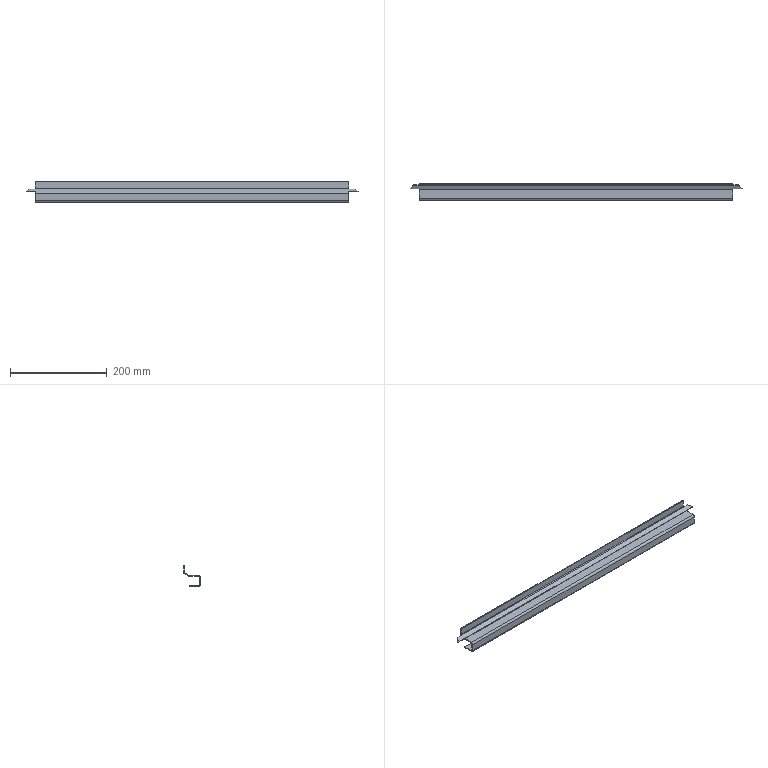Part | NX | features solid 2 | 1 solid | 30 faces | box 687.942 x 35 x 43 mm | volume 117426 mm3 | plane 22 | cylinder 8 | commonest cylinder face diameters 4 x4 8 x4
STEP:
#1=CARTESIAN_POINT('',(1221.029,-650.337,635.595));
#2=VERTEX_POINT('',#1);
#3=CARTESIAN_POINT('',(1228.453,-642.211,639.658));
#4=VERTEX_POINT('',#3);
#5=CARTESIAN_POINT('',(1221.029,-650.337,635.595));
#6=DIRECTION('',(0.6327,0.6926,0.3463));
#7=VECTOR('',#6,1000.);
#8=LINE('',#5,#7);
#9=EDGE_CURVE('',#2,#4,#8,.T.);
#10=ORIENTED_EDGE('',*,*,#9,.F.);
#11=CARTESIAN_POINT('',(1221.029,-651.231,637.384));
#12=VERTEX_POINT('',#11);
#13=CARTESIAN_POINT('',(1221.029,-651.231,637.384));
#14=DIRECTION('',(0.,0.4472,-0.8944));
#15=VECTOR('',#14,1000.);
#16=LINE('',#13,#15);
#17=EDGE_CURVE('',#12,#2,#16,.T.);
#18=ORIENTED_EDGE('',*,*,#17,.F.);
#19=CARTESIAN_POINT('',(1228.453,-643.106,641.447));
#20=VERTEX_POINT('',#19);
#21=CARTESIAN_POINT('',(1221.029,-651.231,637.384));
#22=DIRECTION('',(0.6327,0.6926,0.3463));
#23=VECTOR('',#22,1000.);
#24=LINE('',#21,#23);
#25=EDGE_CURVE('',#12,#20,#24,.T.);
#26=ORIENTED_EDGE('',*,*,#25,.T.);
#27=CARTESIAN_POINT('',(1228.453,-643.106,641.447));
#28=DIRECTION('',(0.,0.4472,-0.8944));
#29=VECTOR('',#28,1000.);
#30=LINE('',#27,#29);
#31=EDGE_CURVE('',#20,#4,#30,.T.);
#32=ORIENTED_EDGE('',*,*,#31,.T.);
#33=EDGE_LOOP('',(#10,#18,#26,#32));
#34=FACE_BOUND('',#33,.T.);
#35=CARTESIAN_POINT('',(1221.029,-651.231,637.384));
#36=DIRECTION('',(-0.7744,0.5659,0.283));
#37=DIRECTION('',(0.3432,0.,0.9393));
#38=AXIS2_PLACEMENT_3D('',#35,#36,#37);
#39=PLANE('',#38);
#40=ADVANCED_FACE('',(#34),#39,.T.);
#41=CARTESIAN_POINT('',(1240.,-650.337,635.595));
#42=VERTEX_POINT('',#41);
#43=CARTESIAN_POINT('',(1240.,-650.337,635.595));
#44=DIRECTION('',(-1.,0.,0.));
#45=VECTOR('',#44,1000.);
#46=LINE('',#43,#45);
#47=EDGE_CURVE('',#42,#2,#46,.T.);
#48=ORIENTED_EDGE('',*,*,#47,.F.);
#49=CARTESIAN_POINT('',(1240.,-651.231,637.384));
#50=VERTEX_POINT('',#49);
#51=CARTESIAN_POINT('',(1240.,-651.231,637.384));
#52=DIRECTION('',(0.,0.4472,-0.8944));
#53=VECTOR('',#52,1000.);
#54=LINE('',#51,#53);
#55=EDGE_CURVE('',#50,#42,#54,.T.);
#56=ORIENTED_EDGE('',*,*,#55,.F.);
#57=CARTESIAN_POINT('',(1240.,-651.231,637.384));
#58=DIRECTION('',(-1.,0.,0.));
#59=VECTOR('',#58,1000.);
#60=LINE('',#57,#59);
#61=EDGE_CURVE('',#50,#12,#60,.T.);
#62=ORIENTED_EDGE('',*,*,#61,.T.);
#63=ORIENTED_EDGE('',*,*,#17,.T.);
#64=EDGE_LOOP('',(#48,#56,#62,#63));
#65=FACE_BOUND('',#64,.T.);
#66=CARTESIAN_POINT('',(1240.,-651.231,637.384));
#67=DIRECTION('',(0.,-0.8944,-0.4472));
#68=DIRECTION('',(0.,0.4472,-0.8944));
#69=AXIS2_PLACEMENT_3D('',#66,#67,#68);
#70=PLANE('',#69);
#71=ADVANCED_FACE('',(#65),#70,.T.);
#72=CARTESIAN_POINT('',(1240.,-642.211,639.658));
#73=VERTEX_POINT('',#72);
#74=CARTESIAN_POINT('',(1228.453,-642.211,639.658));
#75=DIRECTION('',(1.,0.,0.));
#76=VECTOR('',#75,1000.);
#77=LINE('',#74,#76);
#78=EDGE_CURVE('',#4,#73,#77,.T.);
#79=ORIENTED_EDGE('',*,*,#78,.F.);
#80=ORIENTED_EDGE('',*,*,#31,.F.);
#81=CARTESIAN_POINT('',(1240.,-643.106,641.447));
#82=VERTEX_POINT('',#81);
#83=CARTESIAN_POINT('',(1228.453,-643.106,641.447));
#84=DIRECTION('',(1.,0.,0.));
#85=VECTOR('',#84,1000.);
#86=LINE('',#83,#85);
#87=EDGE_CURVE('',#20,#82,#86,.T.);
#88=ORIENTED_EDGE('',*,*,#87,.T.);
#89=CARTESIAN_POINT('',(1240.,-643.106,641.447));
#90=DIRECTION('',(0.,0.4472,-0.8944));
#91=VECTOR('',#90,1000.);
#92=LINE('',#89,#91);
#93=EDGE_CURVE('',#82,#73,#92,.T.);
#94=ORIENTED_EDGE('',*,*,#93,.T.);
#95=EDGE_LOOP('',(#79,#80,#88,#94));
#96=FACE_BOUND('',#95,.T.);
#97=CARTESIAN_POINT('',(1228.453,-643.106,641.447));
#98=DIRECTION('',(0.,0.8944,0.4472));
#99=DIRECTION('',(1.,0.,0.));
#100=AXIS2_PLACEMENT_3D('',#97,#98,#99);
#101=PLANE('',#100);
#102=ADVANCED_FACE('',(#96),#101,.T.);
#103=CARTESIAN_POINT('',(1908.971,-650.337,635.595));
#104=VERTEX_POINT('',#103);
#105=CARTESIAN_POINT('',(1890.,-650.337,635.595));
#106=VERTEX_POINT('',#105);
#107=CARTESIAN_POINT('',(1908.971,-650.337,635.595));
#108=DIRECTION('',(-1.,0.,0.));
#109=VECTOR('',#108,1000.);
#110=LINE('',#107,#109);
#111=EDGE_CURVE('',#104,#106,#110,.T.);
#112=ORIENTED_EDGE('',*,*,#111,.F.);
#113=CARTESIAN_POINT('',(1908.971,-651.231,637.384));
#114=VERTEX_POINT('',#113);
#115=CARTESIAN_POINT('',(1908.971,-651.231,637.384));
#116=DIRECTION('',(0.,0.4472,-0.8944));
#117=VECTOR('',#116,1000.);
#118=LINE('',#115,#117);
#119=EDGE_CURVE('',#114,#104,#118,.T.);
#120=ORIENTED_EDGE('',*,*,#119,.F.);
#121=CARTESIAN_POINT('',(1890.,-651.231,637.384));
#122=VERTEX_POINT('',#121);
#123=CARTESIAN_POINT('',(1908.971,-651.231,637.384));
#124=DIRECTION('',(-1.,0.,0.));
#125=VECTOR('',#124,1000.);
#126=LINE('',#123,#125);
#127=EDGE_CURVE('',#114,#122,#126,.T.);
#128=ORIENTED_EDGE('',*,*,#127,.T.);
#129=CARTESIAN_POINT('',(1890.,-651.231,637.384));
#130=DIRECTION('',(0.,0.4472,-0.8944));
#131=VECTOR('',#130,1000.);
#132=LINE('',#129,#131);
#133=EDGE_CURVE('',#122,#106,#132,.T.);
#134=ORIENTED_EDGE('',*,*,#133,.T.);
#135=EDGE_LOOP('',(#112,#120,#128,#134));
#136=FACE_BOUND('',#135,.T.);
#137=CARTESIAN_POINT('',(1908.971,-651.231,637.384));
#138=DIRECTION('',(0.,-0.8944,-0.4472));
#139=DIRECTION('',(0.,0.4472,-0.8944));
#140=AXIS2_PLACEMENT_3D('',#137,#138,#139);
#141=PLANE('',#140);
#142=ADVANCED_FACE('',(#136),#141,.T.);
#143=CARTESIAN_POINT('',(1901.547,-642.211,639.658));
#144=VERTEX_POINT('',#143);
#145=CARTESIAN_POINT('',(1908.971,-650.337,635.595));
#146=DIRECTION('',(0.6327,-0.6926,-0.3463));
#147=VECTOR('',#146,1000.);
#148=LINE('',#145,#147);
#149=EDGE_CURVE('',#144,#104,#148,.T.);
#150=ORIENTED_EDGE('',*,*,#149,.F.);
#151=CARTESIAN_POINT('',(1901.547,-643.106,641.447));
#152=VERTEX_POINT('',#151);
#153=CARTESIAN_POINT('',(1901.547,-643.106,641.447));
#154=DIRECTION('',(0.,0.4472,-0.8944));
#155=VECTOR('',#154,1000.);
#156=LINE('',#153,#155);
#157=EDGE_CURVE('',#152,#144,#156,.T.);
#158=ORIENTED_EDGE('',*,*,#157,.F.);
#159=CARTESIAN_POINT('',(1908.971,-651.231,637.384));
#160=DIRECTION('',(0.6327,-0.6926,-0.3463));
#161=VECTOR('',#160,1000.);
#162=LINE('',#159,#161);
#163=EDGE_CURVE('',#152,#114,#162,.T.);
#164=ORIENTED_EDGE('',*,*,#163,.T.);
#165=ORIENTED_EDGE('',*,*,#119,.T.);
#166=EDGE_LOOP('',(#150,#158,#164,#165));
#167=FACE_BOUND('',#166,.T.);
#168=CARTESIAN_POINT('',(1908.971,-651.231,637.384));
#169=DIRECTION('',(0.7744,0.5659,0.283));
#170=DIRECTION('',(0.,0.4472,-0.8944));
#171=AXIS2_PLACEMENT_3D('',#168,#169,#170);
#172=PLANE('',#171);
#173=ADVANCED_FACE('',(#167),#172,.T.);
#174=CARTESIAN_POINT('',(1890.,-642.211,639.658));
#175=VERTEX_POINT('',#174);
#176=CARTESIAN_POINT('',(1890.,-642.211,639.658));
#177=DIRECTION('',(1.,0.,0.));
#178=VECTOR('',#177,1000.);
#179=LINE('',#176,#178);
#180=EDGE_CURVE('',#175,#144,#179,.T.);
#181=ORIENTED_EDGE('',*,*,#180,.F.);
#182=CARTESIAN_POINT('',(1890.,-643.106,641.447));
#183=VERTEX_POINT('',#182);
#184=CARTESIAN_POINT('',(1890.,-643.106,641.447));
#185=DIRECTION('',(0.,0.4472,-0.8944));
#186=VECTOR('',#185,1000.);
#187=LINE('',#184,#186);
#188=EDGE_CURVE('',#183,#175,#187,.T.);
#189=ORIENTED_EDGE('',*,*,#188,.F.);
#190=CARTESIAN_POINT('',(1890.,-643.106,641.447));
#191=DIRECTION('',(1.,0.,0.));
#192=VECTOR('',#191,1000.);
#193=LINE('',#190,#192);
#194=EDGE_CURVE('',#183,#152,#193,.T.);
#195=ORIENTED_EDGE('',*,*,#194,.T.);
#196=ORIENTED_EDGE('',*,*,#157,.T.);
#197=EDGE_LOOP('',(#181,#189,#195,#196));
#198=FACE_BOUND('',#197,.T.);
#199=CARTESIAN_POINT('',(1890.,-643.106,641.447));
#200=DIRECTION('',(0.,0.8944,0.4472));
#201=DIRECTION('',(1.,0.,0.));
#202=AXIS2_PLACEMENT_3D('',#199,#200,#201);
#203=PLANE('',#202);
#204=ADVANCED_FACE('',(#198),#203,.T.);
#205=CARTESIAN_POINT('',(1240.,-652.472,637.));
#206=VERTEX_POINT('',#205);
#207=CARTESIAN_POINT('',(1890.,-652.472,637.));
#208=VERTEX_POINT('',#207);
#209=CARTESIAN_POINT('',(1240.,-652.472,637.));
#210=DIRECTION('',(1.,0.,0.));
#211=VECTOR('',#210,1000.);
#212=LINE('',#209,#211);
#213=EDGE_CURVE('',#206,#208,#212,.T.);
#214=ORIENTED_EDGE('',*,*,#213,.T.);
#215=CARTESIAN_POINT('',(1890.,-651.578,637.211));
#216=VERTEX_POINT('',#215);
#217=CARTESIAN_POINT('',(1890.,-652.472,639.));
#218=DIRECTION('',(-1.,0.,0.));
#219=DIRECTION('',(0.,1.,0.));
#220=AXIS2_PLACEMENT_3D('',#217,#218,#219);
#221=CIRCLE('',#220,2.);
#222=EDGE_CURVE('',#216,#208,#221,.T.);
#223=ORIENTED_EDGE('',*,*,#222,.F.);
#224=CARTESIAN_POINT('',(1240.,-651.578,637.211));
#225=VERTEX_POINT('',#224);
#226=CARTESIAN_POINT('',(1240.,-651.578,637.211));
#227=DIRECTION('',(1.,0.,0.));
#228=VECTOR('',#227,1000.);
#229=LINE('',#226,#228);
#230=EDGE_CURVE('',#225,#216,#229,.T.);
#231=ORIENTED_EDGE('',*,*,#230,.F.);
#232=CARTESIAN_POINT('',(1240.,-652.472,639.));
#233=DIRECTION('',(-1.,0.,0.));
#234=DIRECTION('',(0.,1.,0.));
#235=AXIS2_PLACEMENT_3D('',#232,#233,#234);
#236=CIRCLE('',#235,2.);
#237=EDGE_CURVE('',#225,#206,#236,.T.);
#238=ORIENTED_EDGE('',*,*,#237,.T.);
#239=EDGE_LOOP('',(#214,#223,#231,#238));
#240=FACE_BOUND('',#239,.T.);
#241=CARTESIAN_POINT('',(1240.,-652.472,639.));
#242=DIRECTION('',(1.,0.,0.));
#243=DIRECTION('',(0.,0.,1.));
#244=AXIS2_PLACEMENT_3D('',#241,#242,#243);
#245=CYLINDRICAL_SURFACE('',#244,2.);
#246=ADVANCED_FACE('',(#240),#245,.F.);
#247=CARTESIAN_POINT('',(1240.,-652.472,635.));
#248=VERTEX_POINT('',#247);
#249=CARTESIAN_POINT('',(1890.,-652.472,635.));
#250=VERTEX_POINT('',#249);
#251=CARTESIAN_POINT('',(1240.,-652.472,635.));
#252=DIRECTION('',(1.,0.,0.));
#253=VECTOR('',#252,1000.);
#254=LINE('',#251,#253);
#255=EDGE_CURVE('',#248,#250,#254,.T.);
#256=ORIENTED_EDGE('',*,*,#255,.F.);
#257=CARTESIAN_POINT('',(1240.,-650.683,635.422));
#258=VERTEX_POINT('',#257);
#259=CARTESIAN_POINT('',(1240.,-652.472,639.));
#260=DIRECTION('',(-1.,0.,0.));
#261=DIRECTION('',(0.,0.,1.));
#262=AXIS2_PLACEMENT_3D('',#259,#260,#261);
#263=CIRCLE('',#262,4.);
#264=EDGE_CURVE('',#258,#248,#263,.T.);
#265=ORIENTED_EDGE('',*,*,#264,.F.);
#266=CARTESIAN_POINT('',(1890.,-650.683,635.422));
#267=VERTEX_POINT('',#266);
#268=CARTESIAN_POINT('',(1240.,-650.683,635.422));
#269=DIRECTION('',(1.,0.,0.));
#270=VECTOR('',#269,1000.);
#271=LINE('',#268,#270);
#272=EDGE_CURVE('',#258,#267,#271,.T.);
#273=ORIENTED_EDGE('',*,*,#272,.T.);
#274=CARTESIAN_POINT('',(1890.,-652.472,639.));
#275=DIRECTION('',(-1.,0.,0.));
#276=DIRECTION('',(0.,0.,1.));
#277=AXIS2_PLACEMENT_3D('',#274,#275,#276);
#278=CIRCLE('',#277,4.);
#279=EDGE_CURVE('',#267,#250,#278,.T.);
#280=ORIENTED_EDGE('',*,*,#279,.T.);
#281=EDGE_LOOP('',(#256,#265,#273,#280));
#282=FACE_BOUND('',#281,.T.);
#283=CARTESIAN_POINT('',(1240.,-652.472,639.));
#284=DIRECTION('',(1.,0.,0.));
#285=DIRECTION('',(0.,0.,1.));
#286=AXIS2_PLACEMENT_3D('',#283,#284,#285);
#287=CYLINDRICAL_SURFACE('',#286,4.);
#288=ADVANCED_FACE('',(#282),#287,.T.);
#289=CARTESIAN_POINT('',(1890.,-640.,643.236));
#290=VERTEX_POINT('',#289);
#291=CARTESIAN_POINT('',(1890.,-640.,657.));
#292=VERTEX_POINT('',#291);
#293=CARTESIAN_POINT('',(1890.,-640.,642.));
#294=DIRECTION('',(0.,0.,1.));
#295=VECTOR('',#294,1000.);
#296=LINE('',#293,#295);
#297=EDGE_CURVE('',#290,#292,#296,.T.);
#298=ORIENTED_EDGE('',*,*,#297,.F.);
#299=CARTESIAN_POINT('',(1240.,-640.,643.236));
#300=VERTEX_POINT('',#299);
#301=CARTESIAN_POINT('',(1240.,-640.,643.236));
#302=DIRECTION('',(1.,0.,0.));
#303=VECTOR('',#302,1000.);
#304=LINE('',#301,#303);
#305=EDGE_CURVE('',#300,#290,#304,.T.);
#306=ORIENTED_EDGE('',*,*,#305,.F.);
#307=CARTESIAN_POINT('',(1240.,-640.,657.));
#308=VERTEX_POINT('',#307);
#309=CARTESIAN_POINT('',(1240.,-640.,642.));
#310=DIRECTION('',(0.,0.,1.));
#311=VECTOR('',#310,1000.);
#312=LINE('',#309,#311);
#313=EDGE_CURVE('',#300,#308,#312,.T.);
#314=ORIENTED_EDGE('',*,*,#313,.T.);
#315=CARTESIAN_POINT('',(1240.,-640.,657.));
#316=DIRECTION('',(1.,0.,0.));
#317=VECTOR('',#316,1000.);
#318=LINE('',#315,#317);
#319=EDGE_CURVE('',#308,#292,#318,.T.);
#320=ORIENTED_EDGE('',*,*,#319,.T.);
#321=EDGE_LOOP('',(#298,#306,#314,#320));
#322=FACE_BOUND('',#321,.T.);
#323=CARTESIAN_POINT('',(1240.,-640.,642.));
#324=DIRECTION('',(0.,1.,0.));
#325=DIRECTION('',(0.,0.,-1.));
#326=AXIS2_PLACEMENT_3D('',#323,#324,#325);
#327=PLANE('',#326);
#328=ADVANCED_FACE('',(#322),#327,.T.);
#329=CARTESIAN_POINT('',(1890.,-644.,643.236));
#330=DIRECTION('',(1.,0.,0.));
#331=DIRECTION('',(0.,1.,0.));
#332=AXIS2_PLACEMENT_3D('',#329,#330,#331);
#333=CIRCLE('',#332,4.);
#334=EDGE_CURVE('',#175,#290,#333,.T.);
#335=ORIENTED_EDGE('',*,*,#334,.F.);
#336=CARTESIAN_POINT('',(1240.,-642.211,639.658));
#337=DIRECTION('',(1.,0.,0.));
#338=VECTOR('',#337,1000.);
#339=LINE('',#336,#338);
#340=EDGE_CURVE('',#73,#175,#339,.T.);
#341=ORIENTED_EDGE('',*,*,#340,.F.);
#342=CARTESIAN_POINT('',(1240.,-644.,643.236));
#343=DIRECTION('',(1.,0.,0.));
#344=DIRECTION('',(0.,1.,0.));
#345=AXIS2_PLACEMENT_3D('',#342,#343,#344);
#346=CIRCLE('',#345,4.);
#347=EDGE_CURVE('',#73,#300,#346,.T.);
#348=ORIENTED_EDGE('',*,*,#347,.T.);
#349=ORIENTED_EDGE('',*,*,#305,.T.);
#350=EDGE_LOOP('',(#335,#341,#348,#349));
#351=FACE_BOUND('',#350,.T.);
#352=CARTESIAN_POINT('',(1240.,-644.,643.236));
#353=DIRECTION('',(1.,0.,0.));
#354=DIRECTION('',(0.,1.,0.));
#355=AXIS2_PLACEMENT_3D('',#352,#353,#354);
#356=CYLINDRICAL_SURFACE('',#355,4.);
#357=ADVANCED_FACE('',(#351),#356,.T.);
#358=CARTESIAN_POINT('',(1890.,-651.106,635.211));
#359=DIRECTION('',(0.,0.8944,0.4472));
#360=VECTOR('',#359,1000.);
#361=LINE('',#358,#360);
#362=EDGE_CURVE('',#267,#106,#361,.T.);
#363=ORIENTED_EDGE('',*,*,#362,.F.);
#364=ORIENTED_EDGE('',*,*,#272,.F.);
#365=CARTESIAN_POINT('',(1240.,-651.106,635.211));
#366=DIRECTION('',(0.,0.8944,0.4472));
#367=VECTOR('',#366,1000.);
#368=LINE('',#365,#367);
#369=EDGE_CURVE('',#258,#42,#368,.T.);
#370=ORIENTED_EDGE('',*,*,#369,.T.);
#371=ORIENTED_EDGE('',*,*,#47,.T.);
#372=ORIENTED_EDGE('',*,*,#9,.T.);
#373=ORIENTED_EDGE('',*,*,#78,.T.);
#374=ORIENTED_EDGE('',*,*,#340,.T.);
#375=ORIENTED_EDGE('',*,*,#180,.T.);
#376=ORIENTED_EDGE('',*,*,#149,.T.);
#377=ORIENTED_EDGE('',*,*,#111,.T.);
#378=EDGE_LOOP('',(#363,#364,#370,#371,#372,#373,#374,#375,#376,#377));
#379=FACE_BOUND('',#378,.T.);
#380=CARTESIAN_POINT('',(1240.,-651.106,635.211));
#381=DIRECTION('',(0.,0.4472,-0.8944));
#382=DIRECTION('',(-1.,0.,0.));
#383=AXIS2_PLACEMENT_3D('',#380,#381,#382);
#384=PLANE('',#383);
#385=ADVANCED_FACE('',(#379),#384,.T.);
#386=CARTESIAN_POINT('',(1890.,-642.,643.236));
#387=VERTEX_POINT('',#386);
#388=CARTESIAN_POINT('',(1890.,-642.,657.));
#389=VERTEX_POINT('',#388);
#390=CARTESIAN_POINT('',(1890.,-642.,642.));
#391=DIRECTION('',(0.,0.,1.));
#392=VECTOR('',#391,1000.);
#393=LINE('',#390,#392);
#394=EDGE_CURVE('',#387,#389,#393,.T.);
#395=ORIENTED_EDGE('',*,*,#394,.T.);
#396=CARTESIAN_POINT('',(1240.,-642.,657.));
#397=VERTEX_POINT('',#396);
#398=CARTESIAN_POINT('',(1240.,-642.,657.));
#399=DIRECTION('',(1.,0.,0.));
#400=VECTOR('',#399,1000.);
#401=LINE('',#398,#400);
#402=EDGE_CURVE('',#397,#389,#401,.T.);
#403=ORIENTED_EDGE('',*,*,#402,.F.);
#404=CARTESIAN_POINT('',(1240.,-642.,643.236));
#405=VERTEX_POINT('',#404);
#406=CARTESIAN_POINT('',(1240.,-642.,642.));
#407=DIRECTION('',(0.,0.,1.));
#408=VECTOR('',#407,1000.);
#409=LINE('',#406,#408);
#410=EDGE_CURVE('',#405,#397,#409,.T.);
#411=ORIENTED_EDGE('',*,*,#410,.F.);
#412=CARTESIAN_POINT('',(1240.,-642.,643.236));
#413=DIRECTION('',(1.,0.,0.));
#414=VECTOR('',#413,1000.);
#415=LINE('',#412,#414);
#416=EDGE_CURVE('',#405,#387,#415,.T.);
#417=ORIENTED_EDGE('',*,*,#416,.T.);
#418=EDGE_LOOP('',(#395,#403,#411,#417));
#419=FACE_BOUND('',#418,.T.);
#420=CARTESIAN_POINT('',(1240.,-642.,642.));
#421=DIRECTION('',(0.,1.,0.));
#422=DIRECTION('',(0.,0.,-1.));
#423=AXIS2_PLACEMENT_3D('',#420,#421,#422);
#424=PLANE('',#423);
#425=ADVANCED_FACE('',(#419),#424,.F.);
#426=CARTESIAN_POINT('',(1890.,-644.,643.236));
#427=DIRECTION('',(1.,0.,0.));
#428=DIRECTION('',(0.,-1.,0.));
#429=AXIS2_PLACEMENT_3D('',#426,#427,#428);
#430=CIRCLE('',#429,2.);
#431=EDGE_CURVE('',#183,#387,#430,.T.);
#432=ORIENTED_EDGE('',*,*,#431,.T.);
#433=ORIENTED_EDGE('',*,*,#416,.F.);
#434=CARTESIAN_POINT('',(1240.,-644.,643.236));
#435=DIRECTION('',(1.,0.,0.));
#436=DIRECTION('',(0.,-1.,0.));
#437=AXIS2_PLACEMENT_3D('',#434,#435,#436);
#438=CIRCLE('',#437,2.);
#439=EDGE_CURVE('',#82,#405,#438,.T.);
#440=ORIENTED_EDGE('',*,*,#439,.F.);
#441=CARTESIAN_POINT('',(1240.,-643.106,641.447));
#442=DIRECTION('',(1.,0.,0.));
#443=VECTOR('',#442,1000.);
#444=LINE('',#441,#443);
#445=EDGE_CURVE('',#82,#183,#444,.T.);
#446=ORIENTED_EDGE('',*,*,#445,.T.);
#447=EDGE_LOOP('',(#432,#433,#440,#446));
#448=FACE_BOUND('',#447,.T.);
#449=CARTESIAN_POINT('',(1240.,-644.,643.236));
#450=DIRECTION('',(1.,0.,0.));
#451=DIRECTION('',(0.,1.,0.));
#452=AXIS2_PLACEMENT_3D('',#449,#450,#451);
#453=CYLINDRICAL_SURFACE('',#452,2.);
#454=ADVANCED_FACE('',(#448),#453,.F.);
#455=CARTESIAN_POINT('',(1890.,-652.,637.));
#456=DIRECTION('',(0.,0.8944,0.4472));
#457=VECTOR('',#456,1000.);
#458=LINE('',#455,#457);
#459=EDGE_CURVE('',#216,#122,#458,.T.);
#460=ORIENTED_EDGE('',*,*,#459,.T.);
#461=ORIENTED_EDGE('',*,*,#127,.F.);
#462=ORIENTED_EDGE('',*,*,#163,.F.);
#463=ORIENTED_EDGE('',*,*,#194,.F.);
#464=ORIENTED_EDGE('',*,*,#445,.F.);
#465=ORIENTED_EDGE('',*,*,#87,.F.);
#466=ORIENTED_EDGE('',*,*,#25,.F.);
#467=ORIENTED_EDGE('',*,*,#61,.F.);
#468=CARTESIAN_POINT('',(1240.,-652.,637.));
#469=DIRECTION('',(0.,0.8944,0.4472));
#470=VECTOR('',#469,1000.);
#471=LINE('',#468,#470);
#472=EDGE_CURVE('',#225,#50,#471,.T.);
#473=ORIENTED_EDGE('',*,*,#472,.F.);
#474=ORIENTED_EDGE('',*,*,#230,.T.);
#475=EDGE_LOOP('',(#460,#461,#462,#463,#464,#465,#466,#467,#473,#474));
#476=FACE_BOUND('',#475,.T.);
#477=CARTESIAN_POINT('',(1240.,-652.,637.));
#478=DIRECTION('',(0.,0.4472,-0.8944));
#479=DIRECTION('',(-1.,0.,0.));
#480=AXIS2_PLACEMENT_3D('',#477,#478,#479);
#481=PLANE('',#480);
#482=ADVANCED_FACE('',(#476),#481,.F.);
#483=CARTESIAN_POINT('',(1890.,-642.,657.));
#484=DIRECTION('',(0.,-1.,0.));
#485=VECTOR('',#484,1000.);
#486=LINE('',#483,#485);
#487=EDGE_CURVE('',#292,#389,#486,.T.);
#488=ORIENTED_EDGE('',*,*,#487,.F.);
#489=ORIENTED_EDGE('',*,*,#319,.F.);
#490=CARTESIAN_POINT('',(1240.,-642.,657.));
#491=DIRECTION('',(0.,-1.,0.));
#492=VECTOR('',#491,1000.);
#493=LINE('',#490,#492);
#494=EDGE_CURVE('',#308,#397,#493,.T.);
#495=ORIENTED_EDGE('',*,*,#494,.T.);
#496=ORIENTED_EDGE('',*,*,#402,.T.);
#497=EDGE_LOOP('',(#488,#489,#495,#496));
#498=FACE_BOUND('',#497,.T.);
#499=CARTESIAN_POINT('',(1240.,-642.,657.));
#500=DIRECTION('',(0.,0.,1.));
#501=DIRECTION('',(0.,-1.,0.));
#502=AXIS2_PLACEMENT_3D('',#499,#500,#501);
#503=PLANE('',#502);
#504=ADVANCED_FACE('',(#498),#503,.T.);
#505=CARTESIAN_POINT('',(1240.,-671.,614.));
#506=VERTEX_POINT('',#505);
#507=CARTESIAN_POINT('',(1240.,-652.,614.));
#508=VERTEX_POINT('',#507);
#509=CARTESIAN_POINT('',(1240.,-675.,614.));
#510=DIRECTION('',(0.,1.,0.));
#511=VECTOR('',#510,1000.);
#512=LINE('',#509,#511);
#513=EDGE_CURVE('',#506,#508,#512,.T.);
#514=ORIENTED_EDGE('',*,*,#513,.T.);
#515=CARTESIAN_POINT('',(1890.,-652.,614.));
#516=VERTEX_POINT('',#515);
#517=CARTESIAN_POINT('',(1890.,-652.,614.));
#518=DIRECTION('',(-1.,0.,0.));
#519=VECTOR('',#518,1000.);
#520=LINE('',#517,#519);
#521=EDGE_CURVE('',#516,#508,#520,.T.);
#522=ORIENTED_EDGE('',*,*,#521,.F.);
#523=CARTESIAN_POINT('',(1890.,-671.,614.));
#524=VERTEX_POINT('',#523);
#525=CARTESIAN_POINT('',(1890.,-675.,614.));
#526=DIRECTION('',(0.,1.,0.));
#527=VECTOR('',#526,1000.);
#528=LINE('',#525,#527);
#529=EDGE_CURVE('',#524,#516,#528,.T.);
#530=ORIENTED_EDGE('',*,*,#529,.F.);
#531=CARTESIAN_POINT('',(1890.,-671.,614.));
#532=DIRECTION('',(-1.,0.,0.));
#533=VECTOR('',#532,1000.);
#534=LINE('',#531,#533);
#535=EDGE_CURVE('',#524,#506,#534,.T.);
#536=ORIENTED_EDGE('',*,*,#535,.T.);
#537=EDGE_LOOP('',(#514,#522,#530,#536));
#538=FACE_BOUND('',#537,.T.);
#539=CARTESIAN_POINT('',(1890.,-675.,614.));
#540=DIRECTION('',(0.,0.,1.));
#541=DIRECTION('',(0.,-1.,0.));
#542=AXIS2_PLACEMENT_3D('',#539,#540,#541);
#543=PLANE('',#542);
#544=ADVANCED_FACE('',(#538),#543,.F.);
#545=CARTESIAN_POINT('',(1240.,-675.,618.));
#546=VERTEX_POINT('',#545);
#547=CARTESIAN_POINT('',(1240.,-671.,618.));
#548=DIRECTION('',(1.,0.,0.));
#549=DIRECTION('',(0.,-1.,0.));
#550=AXIS2_PLACEMENT_3D('',#547,#548,#549);
#551=CIRCLE('',#550,4.);
#552=EDGE_CURVE('',#546,#506,#551,.T.);
#553=ORIENTED_EDGE('',*,*,#552,.T.);
#554=ORIENTED_EDGE('',*,*,#535,.F.);
#555=CARTESIAN_POINT('',(1890.,-675.,618.));
#556=VERTEX_POINT('',#555);
#557=CARTESIAN_POINT('',(1890.,-671.,618.));
#558=DIRECTION('',(1.,0.,0.));
#559=DIRECTION('',(0.,-1.,0.));
#560=AXIS2_PLACEMENT_3D('',#557,#558,#559);
#561=CIRCLE('',#560,4.);
#562=EDGE_CURVE('',#556,#524,#561,.T.);
#563=ORIENTED_EDGE('',*,*,#562,.F.);
#564=CARTESIAN_POINT('',(1890.,-675.,618.));
#565=DIRECTION('',(-1.,0.,0.));
#566=VECTOR('',#565,1000.);
#567=LINE('',#564,#566);
#568=EDGE_CURVE('',#556,#546,#567,.T.);
#569=ORIENTED_EDGE('',*,*,#568,.T.);
#570=EDGE_LOOP('',(#553,#554,#563,#569));
#571=FACE_BOUND('',#570,.T.);
#572=CARTESIAN_POINT('',(1890.,-671.,618.));
#573=DIRECTION('',(-1.,0.,0.));
#574=DIRECTION('',(0.,-1.,0.));
#575=AXIS2_PLACEMENT_3D('',#572,#573,#574);
#576=CYLINDRICAL_SURFACE('',#575,4.);
#577=ADVANCED_FACE('',(#571),#576,.T.);
#578=CARTESIAN_POINT('',(1240.,-675.,633.));
#579=VERTEX_POINT('',#578);
#580=CARTESIAN_POINT('',(1240.,-675.,637.));
#581=DIRECTION('',(0.,0.,-1.));
#582=VECTOR('',#581,1000.);
#583=LINE('',#580,#582);
#584=EDGE_CURVE('',#579,#546,#583,.T.);
#585=ORIENTED_EDGE('',*,*,#584,.T.);
#586=ORIENTED_EDGE('',*,*,#568,.F.);
#587=CARTESIAN_POINT('',(1890.,-675.,633.));
#588=VERTEX_POINT('',#587);
#589=CARTESIAN_POINT('',(1890.,-675.,637.));
#590=DIRECTION('',(0.,0.,-1.));
#591=VECTOR('',#590,1000.);
#592=LINE('',#589,#591);
#593=EDGE_CURVE('',#588,#556,#592,.T.);
#594=ORIENTED_EDGE('',*,*,#593,.F.);
#595=CARTESIAN_POINT('',(1890.,-675.,633.));
#596=DIRECTION('',(-1.,0.,0.));
#597=VECTOR('',#596,1000.);
#598=LINE('',#595,#597);
#599=EDGE_CURVE('',#588,#579,#598,.T.);
#600=ORIENTED_EDGE('',*,*,#599,.T.);
#601=EDGE_LOOP('',(#585,#586,#594,#600));
#602=FACE_BOUND('',#601,.T.);
#603=CARTESIAN_POINT('',(1890.,-675.,637.));
#604=DIRECTION('',(0.,1.,0.));
#605=DIRECTION('',(0.,0.,-1.));
#606=AXIS2_PLACEMENT_3D('',#603,#604,#605);
#607=PLANE('',#606);
#608=ADVANCED_FACE('',(#602),#607,.F.);
#609=CARTESIAN_POINT('',(1240.,-671.,637.));
#610=VERTEX_POINT('',#609);
#611=CARTESIAN_POINT('',(1240.,-671.,633.));
#612=DIRECTION('',(1.,0.,0.));
#613=DIRECTION('',(0.,-1.,0.));
#614=AXIS2_PLACEMENT_3D('',#611,#612,#613);
#615=CIRCLE('',#614,4.);
#616=EDGE_CURVE('',#610,#579,#615,.T.);
#617=ORIENTED_EDGE('',*,*,#616,.T.);
#618=ORIENTED_EDGE('',*,*,#599,.F.);
#619=CARTESIAN_POINT('',(1890.,-671.,637.));
#620=VERTEX_POINT('',#619);
#621=CARTESIAN_POINT('',(1890.,-671.,633.));
#622=DIRECTION('',(1.,0.,0.));
#623=DIRECTION('',(0.,-1.,0.));
#624=AXIS2_PLACEMENT_3D('',#621,#622,#623);
#625=CIRCLE('',#624,4.);
#626=EDGE_CURVE('',#620,#588,#625,.T.);
#627=ORIENTED_EDGE('',*,*,#626,.F.);
#628=CARTESIAN_POINT('',(1890.,-671.,637.));
#629=DIRECTION('',(-1.,0.,0.));
#630=VECTOR('',#629,1000.);
#631=LINE('',#628,#630);
#632=EDGE_CURVE('',#620,#610,#631,.T.);
#633=ORIENTED_EDGE('',*,*,#632,.T.);
#634=EDGE_LOOP('',(#617,#618,#627,#633));
#635=FACE_BOUND('',#634,.T.);
#636=CARTESIAN_POINT('',(1890.,-671.,633.));
#637=DIRECTION('',(-1.,0.,0.));
#638=DIRECTION('',(0.,-1.,0.));
#639=AXIS2_PLACEMENT_3D('',#636,#637,#638);
#640=CYLINDRICAL_SURFACE('',#639,4.);
#641=ADVANCED_FACE('',(#635),#640,.T.);
#642=ORIENTED_EDGE('',*,*,#213,.F.);
#643=CARTESIAN_POINT('',(1240.,-652.,637.));
#644=DIRECTION('',(0.,-1.,0.));
#645=VECTOR('',#644,1000.);
#646=LINE('',#643,#645);
#647=EDGE_CURVE('',#206,#610,#646,.T.);
#648=ORIENTED_EDGE('',*,*,#647,.T.);
#649=ORIENTED_EDGE('',*,*,#632,.F.);
#650=CARTESIAN_POINT('',(1890.,-652.,637.));
#651=DIRECTION('',(0.,-1.,0.));
#652=VECTOR('',#651,1000.);
#653=LINE('',#650,#652);
#654=EDGE_CURVE('',#208,#620,#653,.T.);
#655=ORIENTED_EDGE('',*,*,#654,.F.);
#656=EDGE_LOOP('',(#642,#648,#649,#655));
#657=FACE_BOUND('',#656,.T.);
#658=CARTESIAN_POINT('',(1890.,-652.,637.));
#659=DIRECTION('',(0.,0.,-1.));
#660=DIRECTION('',(0.,-1.,0.));
#661=AXIS2_PLACEMENT_3D('',#658,#659,#660);
#662=PLANE('',#661);
#663=ADVANCED_FACE('',(#657),#662,.F.);
#664=CARTESIAN_POINT('',(1240.,-671.,616.));
#665=VERTEX_POINT('',#664);
#666=CARTESIAN_POINT('',(1240.,-652.,616.));
#667=VERTEX_POINT('',#666);
#668=CARTESIAN_POINT('',(1240.,-675.,616.));
#669=DIRECTION('',(0.,1.,0.));
#670=VECTOR('',#669,1000.);
#671=LINE('',#668,#670);
#672=EDGE_CURVE('',#665,#667,#671,.T.);
#673=ORIENTED_EDGE('',*,*,#672,.F.);
#674=CARTESIAN_POINT('',(1890.,-671.,616.));
#675=VERTEX_POINT('',#674);
#676=CARTESIAN_POINT('',(1890.,-671.,616.));
#677=DIRECTION('',(-1.,0.,0.));
#678=VECTOR('',#677,1000.);
#679=LINE('',#676,#678);
#680=EDGE_CURVE('',#675,#665,#679,.T.);
#681=ORIENTED_EDGE('',*,*,#680,.F.);
#682=CARTESIAN_POINT('',(1890.,-652.,616.));
#683=VERTEX_POINT('',#682);
#684=CARTESIAN_POINT('',(1890.,-675.,616.));
#685=DIRECTION('',(0.,1.,0.));
#686=VECTOR('',#685,1000.);
#687=LINE('',#684,#686);
#688=EDGE_CURVE('',#675,#683,#687,.T.);
#689=ORIENTED_EDGE('',*,*,#688,.T.);
#690=CARTESIAN_POINT('',(1890.,-652.,616.));
#691=DIRECTION('',(-1.,0.,0.));
#692=VECTOR('',#691,1000.);
#693=LINE('',#690,#692);
#694=EDGE_CURVE('',#683,#667,#693,.T.);
#695=ORIENTED_EDGE('',*,*,#694,.T.);
#696=EDGE_LOOP('',(#673,#681,#689,#695));
#697=FACE_BOUND('',#696,.T.);
#698=CARTESIAN_POINT('',(1890.,-675.,616.));
#699=DIRECTION('',(0.,0.,1.));
#700=DIRECTION('',(0.,-1.,0.));
#701=AXIS2_PLACEMENT_3D('',#698,#699,#700);
#702=PLANE('',#701);
#703=ADVANCED_FACE('',(#697),#702,.T.);
#704=CARTESIAN_POINT('',(1240.,-673.,618.));
#705=VERTEX_POINT('',#704);
#706=CARTESIAN_POINT('',(1240.,-671.,618.));
#707=DIRECTION('',(1.,0.,0.));
#708=DIRECTION('',(0.,-1.,0.));
#709=AXIS2_PLACEMENT_3D('',#706,#707,#708);
#710=CIRCLE('',#709,2.);
#711=EDGE_CURVE('',#705,#665,#710,.T.);
#712=ORIENTED_EDGE('',*,*,#711,.F.);
#713=CARTESIAN_POINT('',(1890.,-673.,618.));
#714=VERTEX_POINT('',#713);
#715=CARTESIAN_POINT('',(1890.,-673.,618.));
#716=DIRECTION('',(-1.,0.,0.));
#717=VECTOR('',#716,1000.);
#718=LINE('',#715,#717);
#719=EDGE_CURVE('',#714,#705,#718,.T.);
#720=ORIENTED_EDGE('',*,*,#719,.F.);
#721=CARTESIAN_POINT('',(1890.,-671.,618.));
#722=DIRECTION('',(1.,0.,0.));
#723=DIRECTION('',(0.,-1.,0.));
#724=AXIS2_PLACEMENT_3D('',#721,#722,#723);
#725=CIRCLE('',#724,2.);
#726=EDGE_CURVE('',#714,#675,#725,.T.);
#727=ORIENTED_EDGE('',*,*,#726,.T.);
#728=ORIENTED_EDGE('',*,*,#680,.T.);
#729=EDGE_LOOP('',(#712,#720,#727,#728));
#730=FACE_BOUND('',#729,.T.);
#731=CARTESIAN_POINT('',(1890.,-671.,618.));
#732=DIRECTION('',(-1.,0.,0.));
#733=DIRECTION('',(0.,-1.,0.));
#734=AXIS2_PLACEMENT_3D('',#731,#732,#733);
#735=CYLINDRICAL_SURFACE('',#734,2.);
#736=ADVANCED_FACE('',(#730),#735,.F.);
#737=CARTESIAN_POINT('',(1240.,-673.,633.));
#738=VERTEX_POINT('',#737);
#739=CARTESIAN_POINT('',(1240.,-673.,637.));
#740=DIRECTION('',(0.,0.,-1.));
#741=VECTOR('',#740,1000.);
#742=LINE('',#739,#741);
#743=EDGE_CURVE('',#738,#705,#742,.T.);
#744=ORIENTED_EDGE('',*,*,#743,.F.);
#745=CARTESIAN_POINT('',(1890.,-673.,633.));
#746=VERTEX_POINT('',#745);
#747=CARTESIAN_POINT('',(1890.,-673.,633.));
#748=DIRECTION('',(-1.,0.,0.));
#749=VECTOR('',#748,1000.);
#750=LINE('',#747,#749);
#751=EDGE_CURVE('',#746,#738,#750,.T.);
#752=ORIENTED_EDGE('',*,*,#751,.F.);
#753=CARTESIAN_POINT('',(1890.,-673.,637.));
#754=DIRECTION('',(0.,0.,-1.));
#755=VECTOR('',#754,1000.);
#756=LINE('',#753,#755);
#757=EDGE_CURVE('',#746,#714,#756,.T.);
#758=ORIENTED_EDGE('',*,*,#757,.T.);
#759=ORIENTED_EDGE('',*,*,#719,.T.);
#760=EDGE_LOOP('',(#744,#752,#758,#759));
#761=FACE_BOUND('',#760,.T.);
#762=CARTESIAN_POINT('',(1890.,-673.,637.));
#763=DIRECTION('',(0.,1.,0.));
#764=DIRECTION('',(0.,0.,-1.));
#765=AXIS2_PLACEMENT_3D('',#762,#763,#764);
#766=PLANE('',#765);
#767=ADVANCED_FACE('',(#761),#766,.T.);
#768=CARTESIAN_POINT('',(1240.,-671.,635.));
#769=VERTEX_POINT('',#768);
#770=CARTESIAN_POINT('',(1240.,-671.,633.));
#771=DIRECTION('',(1.,0.,0.));
#772=DIRECTION('',(0.,-1.,0.));
#773=AXIS2_PLACEMENT_3D('',#770,#771,#772);
#774=CIRCLE('',#773,2.);
#775=EDGE_CURVE('',#769,#738,#774,.T.);
#776=ORIENTED_EDGE('',*,*,#775,.F.);
#777=CARTESIAN_POINT('',(1890.,-671.,635.));
#778=VERTEX_POINT('',#777);
#779=CARTESIAN_POINT('',(1890.,-671.,635.));
#780=DIRECTION('',(-1.,0.,0.));
#781=VECTOR('',#780,1000.);
#782=LINE('',#779,#781);
#783=EDGE_CURVE('',#778,#769,#782,.T.);
#784=ORIENTED_EDGE('',*,*,#783,.F.);
#785=CARTESIAN_POINT('',(1890.,-671.,633.));
#786=DIRECTION('',(1.,0.,0.));
#787=DIRECTION('',(0.,-1.,0.));
#788=AXIS2_PLACEMENT_3D('',#785,#786,#787);
#789=CIRCLE('',#788,2.);
#790=EDGE_CURVE('',#778,#746,#789,.T.);
#791=ORIENTED_EDGE('',*,*,#790,.T.);
#792=ORIENTED_EDGE('',*,*,#751,.T.);
#793=EDGE_LOOP('',(#776,#784,#791,#792));
#794=FACE_BOUND('',#793,.T.);
#795=CARTESIAN_POINT('',(1890.,-671.,633.));
#796=DIRECTION('',(-1.,0.,0.));
#797=DIRECTION('',(0.,-1.,0.));
#798=AXIS2_PLACEMENT_3D('',#795,#796,#797);
#799=CYLINDRICAL_SURFACE('',#798,2.);
#800=ADVANCED_FACE('',(#794),#799,.F.);
#801=CARTESIAN_POINT('',(1890.,-652.,614.));
#802=DIRECTION('',(0.,0.,1.));
#803=VECTOR('',#802,1000.);
#804=LINE('',#801,#803);
#805=EDGE_CURVE('',#516,#683,#804,.T.);
#806=ORIENTED_EDGE('',*,*,#805,.F.);
#807=ORIENTED_EDGE('',*,*,#521,.T.);
#808=CARTESIAN_POINT('',(1240.,-652.,614.));
#809=DIRECTION('',(0.,0.,1.));
#810=VECTOR('',#809,1000.);
#811=LINE('',#808,#810);
#812=EDGE_CURVE('',#508,#667,#811,.T.);
#813=ORIENTED_EDGE('',*,*,#812,.T.);
#814=ORIENTED_EDGE('',*,*,#694,.F.);
#815=EDGE_LOOP('',(#806,#807,#813,#814));
#816=FACE_BOUND('',#815,.T.);
#817=CARTESIAN_POINT('',(1890.,-652.,614.));
#818=DIRECTION('',(0.,1.,0.));
#819=DIRECTION('',(0.,0.,-1.));
#820=AXIS2_PLACEMENT_3D('',#817,#818,#819);
#821=PLANE('',#820);
#822=ADVANCED_FACE('',(#816),#821,.T.);
#823=CARTESIAN_POINT('',(1240.,-652.,635.));
#824=DIRECTION('',(0.,-1.,0.));
#825=VECTOR('',#824,1000.);
#826=LINE('',#823,#825);
#827=EDGE_CURVE('',#248,#769,#826,.T.);
#828=ORIENTED_EDGE('',*,*,#827,.F.);
#829=ORIENTED_EDGE('',*,*,#255,.T.);
#830=CARTESIAN_POINT('',(1890.,-652.,635.));
#831=DIRECTION('',(0.,-1.,0.));
#832=VECTOR('',#831,1000.);
#833=LINE('',#830,#832);
#834=EDGE_CURVE('',#250,#778,#833,.T.);
#835=ORIENTED_EDGE('',*,*,#834,.T.);
#836=ORIENTED_EDGE('',*,*,#783,.T.);
#837=EDGE_LOOP('',(#828,#829,#835,#836));
#838=FACE_BOUND('',#837,.T.);
#839=CARTESIAN_POINT('',(1890.,-652.,635.));
#840=DIRECTION('',(0.,0.,-1.));
#841=DIRECTION('',(0.,-1.,0.));
#842=AXIS2_PLACEMENT_3D('',#839,#840,#841);
#843=PLANE('',#842);
#844=ADVANCED_FACE('',(#838),#843,.T.);
#845=ORIENTED_EDGE('',*,*,#93,.F.);
#846=ORIENTED_EDGE('',*,*,#439,.T.);
#847=ORIENTED_EDGE('',*,*,#410,.T.);
#848=ORIENTED_EDGE('',*,*,#494,.F.);
#849=ORIENTED_EDGE('',*,*,#313,.F.);
#850=ORIENTED_EDGE('',*,*,#347,.F.);
#851=EDGE_LOOP('',(#845,#846,#847,#848,#849,#850));
#852=FACE_BOUND('',#851,.T.);
#853=CARTESIAN_POINT('',(1240.,-652.,637.));
#854=DIRECTION('',(1.,0.,0.));
#855=DIRECTION('',(0.,0.,1.));
#856=AXIS2_PLACEMENT_3D('',#853,#854,#855);
#857=PLANE('',#856);
#858=ADVANCED_FACE('',(#852),#857,.F.);
#859=ORIENTED_EDGE('',*,*,#133,.F.);
#860=ORIENTED_EDGE('',*,*,#459,.F.);
#861=ORIENTED_EDGE('',*,*,#222,.T.);
#862=ORIENTED_EDGE('',*,*,#654,.T.);
#863=ORIENTED_EDGE('',*,*,#626,.T.);
#864=ORIENTED_EDGE('',*,*,#593,.T.);
#865=ORIENTED_EDGE('',*,*,#562,.T.);
#866=ORIENTED_EDGE('',*,*,#529,.T.);
#867=ORIENTED_EDGE('',*,*,#805,.T.);
#868=ORIENTED_EDGE('',*,*,#688,.F.);
#869=ORIENTED_EDGE('',*,*,#726,.F.);
#870=ORIENTED_EDGE('',*,*,#757,.F.);
#871=ORIENTED_EDGE('',*,*,#790,.F.);
#872=ORIENTED_EDGE('',*,*,#834,.F.);
#873=ORIENTED_EDGE('',*,*,#279,.F.);
#874=ORIENTED_EDGE('',*,*,#362,.T.);
#875=EDGE_LOOP('',(#859,#860,#861,#862,#863,#864,#865,#866,#867,#868,#869,#870,#871,#872,#873,#874));
#876=FACE_BOUND('',#875,.T.);
#877=CARTESIAN_POINT('',(1890.,-675.,614.));
#878=DIRECTION('',(1.,0.,0.));
#879=DIRECTION('',(0.,0.,1.));
#880=AXIS2_PLACEMENT_3D('',#877,#878,#879);
#881=PLANE('',#880);
#882=ADVANCED_FACE('',(#876),#881,.T.);
#883=ORIENTED_EDGE('',*,*,#431,.F.);
#884=ORIENTED_EDGE('',*,*,#188,.T.);
#885=ORIENTED_EDGE('',*,*,#334,.T.);
#886=ORIENTED_EDGE('',*,*,#297,.T.);
#887=ORIENTED_EDGE('',*,*,#487,.T.);
#888=ORIENTED_EDGE('',*,*,#394,.F.);
#889=EDGE_LOOP('',(#883,#884,#885,#886,#887,#888));
#890=FACE_BOUND('',#889,.T.);
#891=CARTESIAN_POINT('',(1890.,-675.,614.));
#892=DIRECTION('',(1.,0.,0.));
#893=DIRECTION('',(0.,0.,1.));
#894=AXIS2_PLACEMENT_3D('',#891,#892,#893);
#895=PLANE('',#894);
#896=ADVANCED_FACE('',(#890),#895,.T.);
#897=ORIENTED_EDGE('',*,*,#472,.T.);
#898=ORIENTED_EDGE('',*,*,#55,.T.);
#899=ORIENTED_EDGE('',*,*,#369,.F.);
#900=ORIENTED_EDGE('',*,*,#264,.T.);
#901=ORIENTED_EDGE('',*,*,#827,.T.);
#902=ORIENTED_EDGE('',*,*,#775,.T.);
#903=ORIENTED_EDGE('',*,*,#743,.T.);
#904=ORIENTED_EDGE('',*,*,#711,.T.);
#905=ORIENTED_EDGE('',*,*,#672,.T.);
#906=ORIENTED_EDGE('',*,*,#812,.F.);
#907=ORIENTED_EDGE('',*,*,#513,.F.);
#908=ORIENTED_EDGE('',*,*,#552,.F.);
#909=ORIENTED_EDGE('',*,*,#584,.F.);
#910=ORIENTED_EDGE('',*,*,#616,.F.);
#911=ORIENTED_EDGE('',*,*,#647,.F.);
#912=ORIENTED_EDGE('',*,*,#237,.F.);
#913=EDGE_LOOP('',(#897,#898,#899,#900,#901,#902,#903,#904,#905,#906,#907,#908,#909,#910,#911,#912));
#914=FACE_BOUND('',#913,.T.);
#915=CARTESIAN_POINT('',(1240.,-652.,637.));
#916=DIRECTION('',(1.,0.,0.));
#917=DIRECTION('',(0.,0.,1.));
#918=AXIS2_PLACEMENT_3D('',#915,#916,#917);
#919=PLANE('',#918);
#920=ADVANCED_FACE('',(#914),#919,.F.);
#921=CLOSED_SHELL('',(#40,#71,#102,#142,#173,#204,#246,#288,#328,#357,#385,#425,#454,#482,#504,#544,#577,#608,#641,#663,#703,#736,#767,#800,#822,#844,#858,#882,#896,#920));
#922=MANIFOLD_SOLID_BREP('',#921);
#923=(LENGTH_UNIT()NAMED_UNIT(*)SI_UNIT(.MILLI.,.METRE.));
#924=UNCERTAINTY_MEASURE_WITH_UNIT(LENGTH_MEASURE(0.00001),#923,'','');
#925=(NAMED_UNIT(*)PLANE_ANGLE_UNIT()SI_UNIT($,.RADIAN.));
#926=(NAMED_UNIT(*)SI_UNIT($,.STERADIAN.)SOLID_ANGLE_UNIT());
#927=(GEOMETRIC_REPRESENTATION_CONTEXT(3)GLOBAL_UNCERTAINTY_ASSIGNED_CONTEXT((#924))GLOBAL_UNIT_ASSIGNED_CONTEXT((#923,#925,#926))REPRESENTATION_CONTEXT('',''));
#928=ADVANCED_BREP_SHAPE_REPRESENTATION('',(#922),#927);